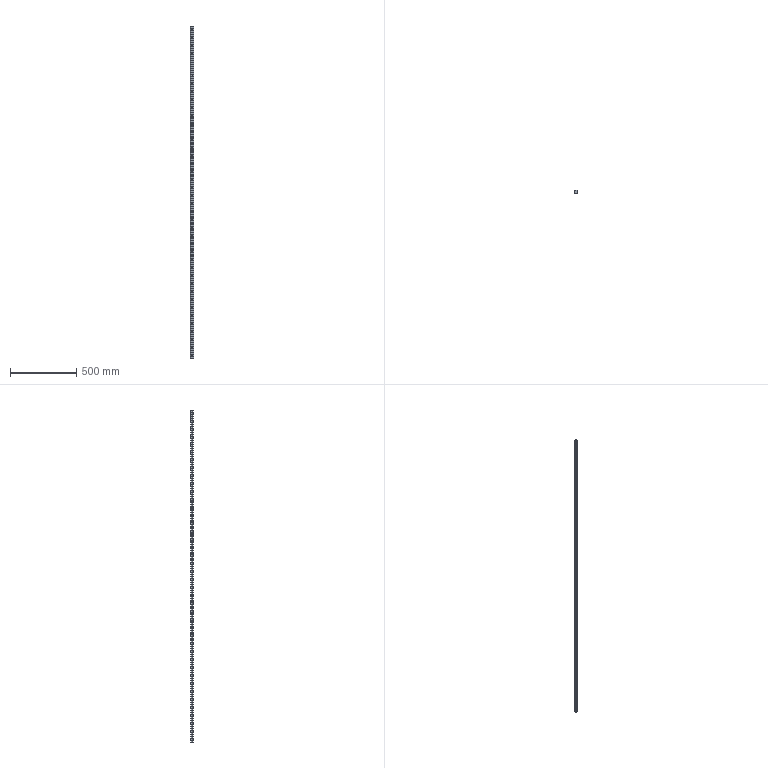Part | STEP file | Linear rail HG25 (HIWIN) | 1 solid | 347 faces | box 23 x 22 x 2500 mm | volume 1042897 mm3 | cylinder 172 | plane 152 | spline 23 | commonest cylinder face diameters 7 x84 11 x84 4.6 x4